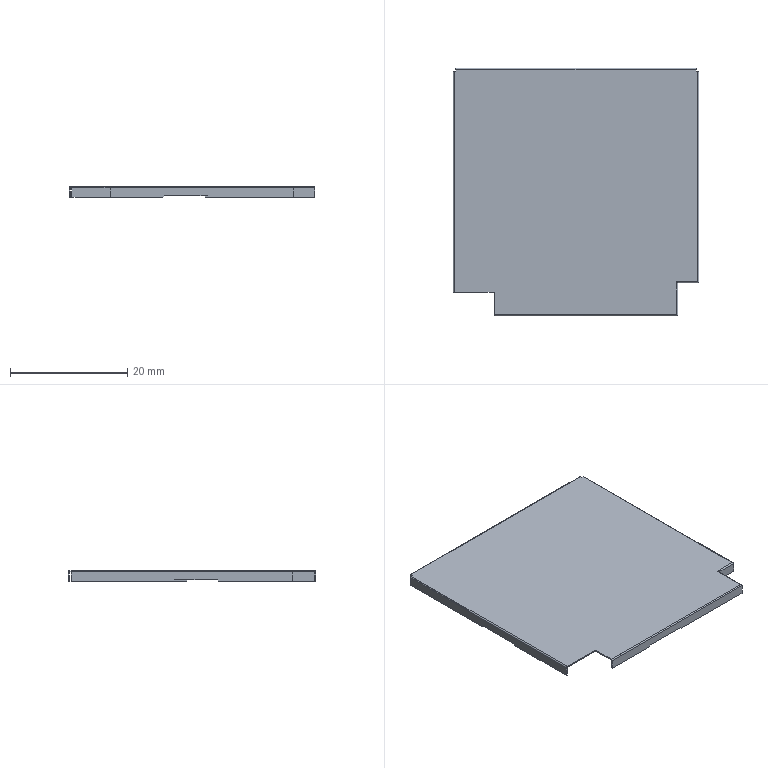Part | Creo | 1 solid | 45 faces | box 41.9 x 42.2 x 1.8 mm | volume 390.663 mm3 | plane 39 | cylinder 6 | commonest cylinder face diameters 0.4 x6
STEP:
#1=CARTESIAN_POINT('',(0.,0.,0.));
#2=DIRECTION('',(0.,0.,1.));
#3=DIRECTION('',(1.,0.,0.));
#4=AXIS2_PLACEMENT_3D('',#1,#2,#3);
#5=CARTESIAN_POINT('',(6.9,0.1,1.8));
#6=VERTEX_POINT('',#5);
#7=CARTESIAN_POINT('',(6.9,3.9,1.8));
#8=VERTEX_POINT('',#7);
#9=CARTESIAN_POINT('',(6.9,0.1,1.8));
#10=DIRECTION('',(0.,1.,0.));
#11=VECTOR('',#10,3.8);
#12=LINE('',#9,#11);
#13=EDGE_CURVE('',#6,#8,#12,.T.);
#14=ORIENTED_EDGE('',*,*,#13,.T.);
#15=CARTESIAN_POINT('',(0.1,3.9,1.8));
#16=VERTEX_POINT('',#15);
#17=CARTESIAN_POINT('',(0.1,3.9,1.8));
#18=DIRECTION('',(1.,0.,0.));
#19=VECTOR('',#18,6.8);
#20=LINE('',#17,#19);
#21=EDGE_CURVE('',#16,#8,#20,.T.);
#22=ORIENTED_EDGE('',*,*,#21,.F.);
#23=CARTESIAN_POINT('',(0.1,41.6,1.8));
#24=VERTEX_POINT('',#23);
#25=CARTESIAN_POINT('',(0.1,41.6,1.8));
#26=DIRECTION('',(0.,-1.,0.));
#27=VECTOR('',#26,37.7);
#28=LINE('',#25,#27);
#29=EDGE_CURVE('',#24,#16,#28,.T.);
#30=ORIENTED_EDGE('',*,*,#29,.F.);
#31=CARTESIAN_POINT('',(0.4,41.6,1.8));
#32=VERTEX_POINT('',#31);
#33=CARTESIAN_POINT('',(0.1,41.6,1.8));
#34=DIRECTION('',(1.,0.,0.));
#35=VECTOR('',#34,0.3);
#36=LINE('',#33,#35);
#37=EDGE_CURVE('',#24,#32,#36,.T.);
#38=ORIENTED_EDGE('',*,*,#37,.T.);
#39=CARTESIAN_POINT('',(0.4,41.9,1.8));
#40=VERTEX_POINT('',#39);
#41=CARTESIAN_POINT('',(0.4,41.9,1.8));
#42=DIRECTION('',(0.,-1.,0.));
#43=VECTOR('',#42,0.3);
#44=LINE('',#41,#43);
#45=EDGE_CURVE('',#40,#32,#44,.T.);
#46=ORIENTED_EDGE('',*,*,#45,.F.);
#47=CARTESIAN_POINT('',(41.3,41.9,1.8));
#48=VERTEX_POINT('',#47);
#49=CARTESIAN_POINT('',(41.3,41.9,1.8));
#50=DIRECTION('',(-1.,0.,0.));
#51=VECTOR('',#50,40.9);
#52=LINE('',#49,#51);
#53=EDGE_CURVE('',#48,#40,#52,.T.);
#54=ORIENTED_EDGE('',*,*,#53,.F.);
#55=CARTESIAN_POINT('',(41.3,41.6,1.8));
#56=VERTEX_POINT('',#55);
#57=CARTESIAN_POINT('',(41.3,41.9,1.8));
#58=DIRECTION('',(0.,-1.,0.));
#59=VECTOR('',#58,0.3);
#60=LINE('',#57,#59);
#61=EDGE_CURVE('',#48,#56,#60,.T.);
#62=ORIENTED_EDGE('',*,*,#61,.T.);
#63=CARTESIAN_POINT('',(41.6,41.6,1.8));
#64=VERTEX_POINT('',#63);
#65=CARTESIAN_POINT('',(41.6,41.6,1.8));
#66=DIRECTION('',(-1.,0.,0.));
#67=VECTOR('',#66,0.3);
#68=LINE('',#65,#67);
#69=EDGE_CURVE('',#64,#56,#68,.T.);
#70=ORIENTED_EDGE('',*,*,#69,.F.);
#71=CARTESIAN_POINT('',(41.6,5.7,1.8));
#72=VERTEX_POINT('',#71);
#73=CARTESIAN_POINT('',(41.6,5.7,1.8));
#74=DIRECTION('',(0.,1.,0.));
#75=VECTOR('',#74,35.9);
#76=LINE('',#73,#75);
#77=EDGE_CURVE('',#72,#64,#76,.T.);
#78=ORIENTED_EDGE('',*,*,#77,.F.);
#79=CARTESIAN_POINT('',(38.,5.7,1.8));
#80=VERTEX_POINT('',#79);
#81=CARTESIAN_POINT('',(38.,5.7,1.8));
#82=DIRECTION('',(1.,0.,0.));
#83=VECTOR('',#82,3.6);
#84=LINE('',#81,#83);
#85=EDGE_CURVE('',#80,#72,#84,.T.);
#86=ORIENTED_EDGE('',*,*,#85,.F.);
#87=CARTESIAN_POINT('',(38.,0.1,1.8));
#88=VERTEX_POINT('',#87);
#89=CARTESIAN_POINT('',(38.,0.1,1.8));
#90=DIRECTION('',(0.,1.,0.));
#91=VECTOR('',#90,5.6);
#92=LINE('',#89,#91);
#93=EDGE_CURVE('',#88,#80,#92,.T.);
#94=ORIENTED_EDGE('',*,*,#93,.F.);
#95=CARTESIAN_POINT('',(6.9,0.1,1.8));
#96=DIRECTION('',(1.,0.,0.));
#97=VECTOR('',#96,31.1);
#98=LINE('',#95,#97);
#99=EDGE_CURVE('',#6,#88,#98,.T.);
#100=ORIENTED_EDGE('',*,*,#99,.F.);
#101=EDGE_LOOP('',(#14,#22,#30,#38,#46,#54,#62,#70,#78,#86,#94,#100));
#102=FACE_OUTER_BOUND('',#101,.F.);
#103=CARTESIAN_POINT('',(0.,0.,1.8));
#104=DIRECTION('',(0.,0.,1.));
#105=DIRECTION('',(1.,0.,0.));
#106=AXIS2_PLACEMENT_3D('',#103,#104,#105);
#107=PLANE('',#106);
#108=ADVANCED_FACE('',(#102),#107,.T.);
#109=CARTESIAN_POINT('',(6.9,-0.1,0.));
#110=VERTEX_POINT('',#109);
#111=CARTESIAN_POINT('',(6.9,0.1,0.));
#112=VERTEX_POINT('',#111);
#113=CARTESIAN_POINT('',(6.9,-0.1,0.));
#114=DIRECTION('',(0.,1.,0.));
#115=VECTOR('',#114,0.2);
#116=LINE('',#113,#115);
#117=EDGE_CURVE('',#110,#112,#116,.T.);
#118=ORIENTED_EDGE('',*,*,#117,.T.);
#119=CARTESIAN_POINT('',(6.9,0.1,1.6));
#120=VERTEX_POINT('',#119);
#121=CARTESIAN_POINT('',(6.9,0.1,0.));
#122=DIRECTION('',(0.,0.,1.));
#123=VECTOR('',#122,1.6);
#124=LINE('',#121,#123);
#125=EDGE_CURVE('',#112,#120,#124,.T.);
#126=ORIENTED_EDGE('',*,*,#125,.T.);
#127=CARTESIAN_POINT('',(6.9,3.9,1.6));
#128=VERTEX_POINT('',#127);
#129=CARTESIAN_POINT('',(6.9,0.1,1.6));
#130=DIRECTION('',(0.,1.,0.));
#131=VECTOR('',#130,3.8);
#132=LINE('',#129,#131);
#133=EDGE_CURVE('',#120,#128,#132,.T.);
#134=ORIENTED_EDGE('',*,*,#133,.T.);
#135=CARTESIAN_POINT('',(6.9,3.9,1.8));
#136=DIRECTION('',(0.,0.,-1.));
#137=VECTOR('',#136,0.2);
#138=LINE('',#135,#137);
#139=EDGE_CURVE('',#8,#128,#138,.T.);
#140=ORIENTED_EDGE('',*,*,#139,.F.);
#141=ORIENTED_EDGE('',*,*,#13,.F.);
#142=CARTESIAN_POINT('',(6.9,-0.1,1.6));
#143=VERTEX_POINT('',#142);
#144=CARTESIAN_POINT('',(6.9,0.1,1.6));
#145=DIRECTION('',(1.,0.,0.));
#146=DIRECTION('',(0.,0.,1.));
#147=AXIS2_PLACEMENT_3D('',#144,#145,#146);
#148=CIRCLE('',#147,0.2);
#149=EDGE_CURVE('',#6,#143,#148,.T.);
#150=ORIENTED_EDGE('',*,*,#149,.T.);
#151=CARTESIAN_POINT('',(6.9,-0.1,0.));
#152=DIRECTION('',(0.,0.,1.));
#153=VECTOR('',#152,1.6);
#154=LINE('',#151,#153);
#155=EDGE_CURVE('',#110,#143,#154,.T.);
#156=ORIENTED_EDGE('',*,*,#155,.F.);
#157=EDGE_LOOP('',(#118,#126,#134,#140,#141,#150,#156));
#158=FACE_OUTER_BOUND('',#157,.F.);
#159=CARTESIAN_POINT('',(6.9,-0.1,1.8));
#160=DIRECTION('',(1.,0.,0.));
#161=DIRECTION('',(0.,1.,0.));
#162=AXIS2_PLACEMENT_3D('',#159,#160,#161);
#163=PLANE('',#162);
#164=ADVANCED_FACE('',(#158),#163,.F.);
#165=ORIENTED_EDGE('',*,*,#117,.F.);
#166=CARTESIAN_POINT('',(15.878,-0.1,0.));
#167=VERTEX_POINT('',#166);
#168=CARTESIAN_POINT('',(6.9,-0.1,0.));
#169=DIRECTION('',(1.,0.,0.));
#170=VECTOR('',#169,8.978);
#171=LINE('',#168,#170);
#172=EDGE_CURVE('',#110,#167,#171,.T.);
#173=ORIENTED_EDGE('',*,*,#172,.T.);
#174=CARTESIAN_POINT('',(15.878,0.1,0.));
#175=VERTEX_POINT('',#174);
#176=CARTESIAN_POINT('',(15.878,0.1,0.));
#177=DIRECTION('',(0.,-1.,0.));
#178=VECTOR('',#177,0.2);
#179=LINE('',#176,#178);
#180=EDGE_CURVE('',#175,#167,#179,.T.);
#181=ORIENTED_EDGE('',*,*,#180,.F.);
#182=CARTESIAN_POINT('',(6.9,0.1,0.));
#183=DIRECTION('',(1.,0.,0.));
#184=VECTOR('',#183,8.978);
#185=LINE('',#182,#184);
#186=EDGE_CURVE('',#112,#175,#185,.T.);
#187=ORIENTED_EDGE('',*,*,#186,.F.);
#188=EDGE_LOOP('',(#165,#173,#181,#187));
#189=FACE_OUTER_BOUND('',#188,.F.);
#190=CARTESIAN_POINT('',(0.,0.,0.));
#191=DIRECTION('',(0.,0.,1.));
#192=DIRECTION('',(1.,0.,0.));
#193=AXIS2_PLACEMENT_3D('',#190,#191,#192);
#194=PLANE('',#193);
#195=ADVANCED_FACE('',(#189),#194,.F.);
#196=ORIENTED_EDGE('',*,*,#155,.T.);
#197=CARTESIAN_POINT('',(38.2,-0.1,1.6));
#198=VERTEX_POINT('',#197);
#199=CARTESIAN_POINT('',(38.2,-0.1,1.6));
#200=DIRECTION('',(-1.,0.,0.));
#201=VECTOR('',#200,31.3);
#202=LINE('',#199,#201);
#203=EDGE_CURVE('',#198,#143,#202,.T.);
#204=ORIENTED_EDGE('',*,*,#203,.F.);
#205=CARTESIAN_POINT('',(38.2,-0.1,0.));
#206=VERTEX_POINT('',#205);
#207=CARTESIAN_POINT('',(38.2,-0.1,0.));
#208=DIRECTION('',(0.,0.,1.));
#209=VECTOR('',#208,1.6);
#210=LINE('',#207,#209);
#211=EDGE_CURVE('',#206,#198,#210,.T.);
#212=ORIENTED_EDGE('',*,*,#211,.F.);
#213=CARTESIAN_POINT('',(23.678,-0.1,0.));
#214=VERTEX_POINT('',#213);
#215=CARTESIAN_POINT('',(23.678,-0.1,0.));
#216=DIRECTION('',(1.,0.,0.));
#217=VECTOR('',#216,14.522);
#218=LINE('',#215,#217);
#219=EDGE_CURVE('',#214,#206,#218,.T.);
#220=ORIENTED_EDGE('',*,*,#219,.F.);
#221=CARTESIAN_POINT('',(23.428,-0.1,0.25));
#222=VERTEX_POINT('',#221);
#223=CARTESIAN_POINT('',(23.678,-0.1,0.));
#224=DIRECTION('',(-0.7071,0.,0.7071));
#225=VECTOR('',#224,0.3536);
#226=LINE('',#223,#225);
#227=EDGE_CURVE('',#214,#222,#226,.T.);
#228=ORIENTED_EDGE('',*,*,#227,.T.);
#229=CARTESIAN_POINT('',(16.128,-0.1,0.25));
#230=VERTEX_POINT('',#229);
#231=CARTESIAN_POINT('',(16.128,-0.1,0.25));
#232=DIRECTION('',(1.,0.,0.));
#233=VECTOR('',#232,7.3);
#234=LINE('',#231,#233);
#235=EDGE_CURVE('',#230,#222,#234,.T.);
#236=ORIENTED_EDGE('',*,*,#235,.F.);
#237=CARTESIAN_POINT('',(16.128,-0.1,0.25));
#238=DIRECTION('',(-0.7071,0.,-0.7071));
#239=VECTOR('',#238,0.3536);
#240=LINE('',#237,#239);
#241=EDGE_CURVE('',#230,#167,#240,.T.);
#242=ORIENTED_EDGE('',*,*,#241,.T.);
#243=ORIENTED_EDGE('',*,*,#172,.F.);
#244=EDGE_LOOP('',(#196,#204,#212,#220,#228,#236,#242,#243));
#245=FACE_OUTER_BOUND('',#244,.F.);
#246=CARTESIAN_POINT('',(-0.1,-0.1,0.));
#247=DIRECTION('',(0.,-1.,0.));
#248=DIRECTION('',(1.,0.,0.));
#249=AXIS2_PLACEMENT_3D('',#246,#247,#248);
#250=PLANE('',#249);
#251=ADVANCED_FACE('',(#245),#250,.T.);
#252=ORIENTED_EDGE('',*,*,#149,.F.);
#253=ORIENTED_EDGE('',*,*,#99,.T.);
#254=CARTESIAN_POINT('',(38.2,-0.1,1.6));
#255=CARTESIAN_POINT('',(38.2,-0.1,1.62));
#256=CARTESIAN_POINT('',(38.194,-0.09426,1.66));
#257=CARTESIAN_POINT('',(38.165,-0.06468,1.72));
#258=CARTESIAN_POINT('',(38.12,-0.02023,1.763));
#259=CARTESIAN_POINT('',(38.072,0.02774,1.79));
#260=CARTESIAN_POINT('',(38.026,0.07447,1.8));
#261=CARTESIAN_POINT('',(38.,0.1,1.8));
#262=B_SPLINE_CURVE_WITH_KNOTS('',3,(#254,#255,#256,#257,#258,#259,#260,#261),.UNSPECIFIED.,.F.,.F.,(4,1,1,1,1,4),(0.,0.2,0.4,0.6,0.8,1.),.UNSPECIFIED.);
#263=EDGE_CURVE('',#198,#88,#262,.T.);
#264=ORIENTED_EDGE('',*,*,#263,.F.);
#265=ORIENTED_EDGE('',*,*,#203,.T.);
#266=EDGE_LOOP('',(#252,#253,#264,#265));
#267=FACE_OUTER_BOUND('',#266,.F.);
#268=CARTESIAN_POINT('',(-55.792,0.1,1.6));
#269=DIRECTION('',(1.,0.,0.));
#270=DIRECTION('',(0.,0.,1.));
#271=AXIS2_PLACEMENT_3D('',#268,#269,#270);
#272=CYLINDRICAL_SURFACE('',#271,0.2);
#273=ADVANCED_FACE('',(#267),#272,.T.);
#274=CARTESIAN_POINT('',(38.2,5.5,1.6));
#275=VERTEX_POINT('',#274);
#276=CARTESIAN_POINT('',(38.2,5.5,1.6));
#277=DIRECTION('',(0.,-1.,0.));
#278=VECTOR('',#277,5.6);
#279=LINE('',#276,#278);
#280=EDGE_CURVE('',#275,#198,#279,.T.);
#281=ORIENTED_EDGE('',*,*,#280,.T.);
#282=ORIENTED_EDGE('',*,*,#263,.T.);
#283=ORIENTED_EDGE('',*,*,#93,.T.);
#284=CARTESIAN_POINT('',(38.2,5.5,1.6));
#285=CARTESIAN_POINT('',(38.2,5.5,1.62));
#286=CARTESIAN_POINT('',(38.194,5.506,1.66));
#287=CARTESIAN_POINT('',(38.165,5.535,1.72));
#288=CARTESIAN_POINT('',(38.12,5.58,1.763));
#289=CARTESIAN_POINT('',(38.072,5.628,1.79));
#290=CARTESIAN_POINT('',(38.026,5.674,1.8));
#291=CARTESIAN_POINT('',(38.,5.7,1.8));
#292=B_SPLINE_CURVE_WITH_KNOTS('',3,(#284,#285,#286,#287,#288,#289,#290,#291),.UNSPECIFIED.,.F.,.F.,(4,1,1,1,1,4),(0.,0.2,0.4,0.6,0.8,1.),.UNSPECIFIED.);
#293=EDGE_CURVE('',#275,#80,#292,.T.);
#294=ORIENTED_EDGE('',*,*,#293,.F.);
#295=EDGE_LOOP('',(#281,#282,#283,#294));
#296=FACE_OUTER_BOUND('',#295,.F.);
#297=CARTESIAN_POINT('',(38.,-56.156,1.6));
#298=DIRECTION('',(0.,1.,0.));
#299=DIRECTION('',(0.,0.,1.));
#300=AXIS2_PLACEMENT_3D('',#297,#298,#299);
#301=CYLINDRICAL_SURFACE('',#300,0.2);
#302=ADVANCED_FACE('',(#296),#301,.T.);
#303=ORIENTED_EDGE('',*,*,#280,.F.);
#304=CARTESIAN_POINT('',(38.2,5.5,0.));
#305=VERTEX_POINT('',#304);
#306=CARTESIAN_POINT('',(38.2,5.5,0.));
#307=DIRECTION('',(0.,0.,1.));
#308=VECTOR('',#307,1.6);
#309=LINE('',#306,#308);
#310=EDGE_CURVE('',#305,#275,#309,.T.);
#311=ORIENTED_EDGE('',*,*,#310,.F.);
#312=CARTESIAN_POINT('',(38.2,-0.1,0.));
#313=DIRECTION('',(0.,1.,0.));
#314=VECTOR('',#313,5.6);
#315=LINE('',#312,#314);
#316=EDGE_CURVE('',#206,#305,#315,.T.);
#317=ORIENTED_EDGE('',*,*,#316,.F.);
#318=ORIENTED_EDGE('',*,*,#211,.T.);
#319=EDGE_LOOP('',(#303,#311,#317,#318));
#320=FACE_OUTER_BOUND('',#319,.F.);
#321=CARTESIAN_POINT('',(38.2,-0.1,0.));
#322=DIRECTION('',(1.,0.,0.));
#323=DIRECTION('',(0.,1.,0.));
#324=AXIS2_PLACEMENT_3D('',#321,#322,#323);
#325=PLANE('',#324);
#326=ADVANCED_FACE('',(#320),#325,.T.);
#327=CARTESIAN_POINT('',(41.8,5.5,1.6));
#328=VERTEX_POINT('',#327);
#329=CARTESIAN_POINT('',(41.8,5.5,1.6));
#330=DIRECTION('',(-1.,0.,0.));
#331=VECTOR('',#330,3.6);
#332=LINE('',#329,#331);
#333=EDGE_CURVE('',#328,#275,#332,.T.);
#334=ORIENTED_EDGE('',*,*,#333,.F.);
#335=CARTESIAN_POINT('',(41.8,5.5,0.));
#336=VERTEX_POINT('',#335);
#337=CARTESIAN_POINT('',(41.8,5.5,0.));
#338=DIRECTION('',(0.,0.,1.));
#339=VECTOR('',#338,1.6);
#340=LINE('',#337,#339);
#341=EDGE_CURVE('',#336,#328,#340,.T.);
#342=ORIENTED_EDGE('',*,*,#341,.F.);
#343=CARTESIAN_POINT('',(38.2,5.5,0.));
#344=DIRECTION('',(1.,0.,0.));
#345=VECTOR('',#344,3.6);
#346=LINE('',#343,#345);
#347=EDGE_CURVE('',#305,#336,#346,.T.);
#348=ORIENTED_EDGE('',*,*,#347,.F.);
#349=ORIENTED_EDGE('',*,*,#310,.T.);
#350=EDGE_LOOP('',(#334,#342,#348,#349));
#351=FACE_OUTER_BOUND('',#350,.F.);
#352=CARTESIAN_POINT('',(38.2,5.5,0.));
#353=DIRECTION('',(0.,-1.,0.));
#354=DIRECTION('',(1.,0.,0.));
#355=AXIS2_PLACEMENT_3D('',#352,#353,#354);
#356=PLANE('',#355);
#357=ADVANCED_FACE('',(#351),#356,.T.);
#358=ORIENTED_EDGE('',*,*,#333,.T.);
#359=ORIENTED_EDGE('',*,*,#293,.T.);
#360=ORIENTED_EDGE('',*,*,#85,.T.);
#361=CARTESIAN_POINT('',(41.8,5.5,1.6));
#362=CARTESIAN_POINT('',(41.8,5.5,1.62));
#363=CARTESIAN_POINT('',(41.794,5.506,1.66));
#364=CARTESIAN_POINT('',(41.765,5.535,1.72));
#365=CARTESIAN_POINT('',(41.72,5.58,1.763));
#366=CARTESIAN_POINT('',(41.672,5.628,1.79));
#367=CARTESIAN_POINT('',(41.626,5.674,1.8));
#368=CARTESIAN_POINT('',(41.6,5.7,1.8));
#369=B_SPLINE_CURVE_WITH_KNOTS('',3,(#361,#362,#363,#364,#365,#366,#367,#368),.UNSPECIFIED.,.F.,.F.,(4,1,1,1,1,4),(0.,0.2,0.4,0.6,0.8,1.),.UNSPECIFIED.);
#370=EDGE_CURVE('',#328,#72,#369,.T.);
#371=ORIENTED_EDGE('',*,*,#370,.F.);
#372=EDGE_LOOP('',(#358,#359,#360,#371));
#373=FACE_OUTER_BOUND('',#372,.F.);
#374=CARTESIAN_POINT('',(-47.321,5.7,1.6));
#375=DIRECTION('',(1.,0.,0.));
#376=DIRECTION('',(0.,0.,1.));
#377=AXIS2_PLACEMENT_3D('',#374,#375,#376);
#378=CYLINDRICAL_SURFACE('',#377,0.2);
#379=ADVANCED_FACE('',(#373),#378,.T.);
#380=CARTESIAN_POINT('',(41.8,41.6,1.6));
#381=VERTEX_POINT('',#380);
#382=CARTESIAN_POINT('',(41.6,41.6,1.6));
#383=DIRECTION('',(0.,-1.,0.));
#384=DIRECTION('',(1.,0.,0.));
#385=AXIS2_PLACEMENT_3D('',#382,#383,#384);
#386=CIRCLE('',#385,0.2);
#387=EDGE_CURVE('',#381,#64,#386,.T.);
#388=ORIENTED_EDGE('',*,*,#387,.F.);
#389=CARTESIAN_POINT('',(41.8,41.6,1.6));
#390=DIRECTION('',(0.,-1.,0.));
#391=VECTOR('',#390,36.1);
#392=LINE('',#389,#391);
#393=EDGE_CURVE('',#381,#328,#392,.T.);
#394=ORIENTED_EDGE('',*,*,#393,.T.);
#395=ORIENTED_EDGE('',*,*,#370,.T.);
#396=ORIENTED_EDGE('',*,*,#77,.T.);
#397=EDGE_LOOP('',(#388,#394,#395,#396));
#398=FACE_OUTER_BOUND('',#397,.F.);
#399=CARTESIAN_POINT('',(41.6,-56.156,1.6));
#400=DIRECTION('',(0.,1.,0.));
#401=DIRECTION('',(0.,0.,1.));
#402=AXIS2_PLACEMENT_3D('',#399,#400,#401);
#403=CYLINDRICAL_SURFACE('',#402,0.2);
#404=ADVANCED_FACE('',(#398),#403,.T.);
#405=CARTESIAN_POINT('',(41.8,41.6,0.));
#406=VERTEX_POINT('',#405);
#407=CARTESIAN_POINT('',(41.6,41.6,0.));
#408=VERTEX_POINT('',#407);
#409=CARTESIAN_POINT('',(41.8,41.6,0.));
#410=DIRECTION('',(-1.,0.,0.));
#411=VECTOR('',#410,0.2);
#412=LINE('',#409,#411);
#413=EDGE_CURVE('',#406,#408,#412,.T.);
#414=ORIENTED_EDGE('',*,*,#413,.F.);
#415=CARTESIAN_POINT('',(41.8,41.6,0.));
#416=DIRECTION('',(0.,0.,1.));
#417=VECTOR('',#416,1.6);
#418=LINE('',#415,#417);
#419=EDGE_CURVE('',#406,#381,#418,.T.);
#420=ORIENTED_EDGE('',*,*,#419,.T.);
#421=ORIENTED_EDGE('',*,*,#387,.T.);
#422=ORIENTED_EDGE('',*,*,#69,.T.);
#423=CARTESIAN_POINT('',(41.3,41.6,1.6));
#424=VERTEX_POINT('',#423);
#425=CARTESIAN_POINT('',(41.3,41.6,1.8));
#426=DIRECTION('',(0.,0.,-1.));
#427=VECTOR('',#426,0.2);
#428=LINE('',#425,#427);
#429=EDGE_CURVE('',#56,#424,#428,.T.);
#430=ORIENTED_EDGE('',*,*,#429,.T.);
#431=CARTESIAN_POINT('',(41.6,41.6,1.6));
#432=VERTEX_POINT('',#431);
#433=CARTESIAN_POINT('',(41.6,41.6,1.6));
#434=DIRECTION('',(-1.,0.,0.));
#435=VECTOR('',#434,0.3);
#436=LINE('',#433,#435);
#437=EDGE_CURVE('',#432,#424,#436,.T.);
#438=ORIENTED_EDGE('',*,*,#437,.F.);
#439=CARTESIAN_POINT('',(41.6,41.6,0.));
#440=DIRECTION('',(0.,0.,1.));
#441=VECTOR('',#440,1.6);
#442=LINE('',#439,#441);
#443=EDGE_CURVE('',#408,#432,#442,.T.);
#444=ORIENTED_EDGE('',*,*,#443,.F.);
#445=EDGE_LOOP('',(#414,#420,#421,#422,#430,#438,#444));
#446=FACE_OUTER_BOUND('',#445,.F.);
#447=CARTESIAN_POINT('',(41.3,41.6,1.8));
#448=DIRECTION('',(0.,-1.,0.));
#449=DIRECTION('',(1.,0.,0.));
#450=AXIS2_PLACEMENT_3D('',#447,#448,#449);
#451=PLANE('',#450);
#452=ADVANCED_FACE('',(#446),#451,.F.);
#453=CARTESIAN_POINT('',(41.8,22.,0.));
#454=VERTEX_POINT('',#453);
#455=CARTESIAN_POINT('',(41.6,22.,0.));
#456=VERTEX_POINT('',#455);
#457=CARTESIAN_POINT('',(41.8,22.,0.));
#458=DIRECTION('',(-1.,0.,0.));
#459=VECTOR('',#458,0.2);
#460=LINE('',#457,#459);
#461=EDGE_CURVE('',#454,#456,#460,.T.);
#462=ORIENTED_EDGE('',*,*,#461,.F.);
#463=CARTESIAN_POINT('',(41.8,22.,0.));
#464=DIRECTION('',(0.,1.,0.));
#465=VECTOR('',#464,19.6);
#466=LINE('',#463,#465);
#467=EDGE_CURVE('',#454,#406,#466,.T.);
#468=ORIENTED_EDGE('',*,*,#467,.T.);
#469=ORIENTED_EDGE('',*,*,#413,.T.);
#470=CARTESIAN_POINT('',(41.6,22.,0.));
#471=DIRECTION('',(0.,1.,0.));
#472=VECTOR('',#471,19.6);
#473=LINE('',#470,#472);
#474=EDGE_CURVE('',#456,#408,#473,.T.);
#475=ORIENTED_EDGE('',*,*,#474,.F.);
#476=EDGE_LOOP('',(#462,#468,#469,#475));
#477=FACE_OUTER_BOUND('',#476,.F.);
#478=CARTESIAN_POINT('',(0.,0.,0.));
#479=DIRECTION('',(0.,0.,1.));
#480=DIRECTION('',(1.,0.,0.));
#481=AXIS2_PLACEMENT_3D('',#478,#479,#480);
#482=PLANE('',#481);
#483=ADVANCED_FACE('',(#477),#482,.F.);
#484=CARTESIAN_POINT('',(41.6,21.75,0.25));
#485=VERTEX_POINT('',#484);
#486=CARTESIAN_POINT('',(41.6,21.75,0.25));
#487=DIRECTION('',(0.,0.7071,-0.7071));
#488=VECTOR('',#487,0.3536);
#489=LINE('',#486,#488);
#490=EDGE_CURVE('',#485,#456,#489,.T.);
#491=ORIENTED_EDGE('',*,*,#490,.F.);
#492=CARTESIAN_POINT('',(41.8,21.75,0.25));
#493=VERTEX_POINT('',#492);
#494=CARTESIAN_POINT('',(41.8,21.75,0.25));
#495=DIRECTION('',(-1.,0.,0.));
#496=VECTOR('',#495,0.2);
#497=LINE('',#494,#496);
#498=EDGE_CURVE('',#493,#485,#497,.T.);
#499=ORIENTED_EDGE('',*,*,#498,.F.);
#500=CARTESIAN_POINT('',(41.8,22.,0.));
#501=DIRECTION('',(0.,-0.7071,0.7071));
#502=VECTOR('',#501,0.3536);
#503=LINE('',#500,#502);
#504=EDGE_CURVE('',#454,#493,#503,.T.);
#505=ORIENTED_EDGE('',*,*,#504,.F.);
#506=ORIENTED_EDGE('',*,*,#461,.T.);
#507=EDGE_LOOP('',(#491,#499,#505,#506));
#508=FACE_OUTER_BOUND('',#507,.F.);
#509=CARTESIAN_POINT('',(41.7,21.875,0.125));
#510=DIRECTION('',(0.,-0.7071,-0.7071));
#511=DIRECTION('',(0.,-0.7071,0.7071));
#512=AXIS2_PLACEMENT_3D('',#509,#510,#511);
#513=PLANE('',#512);
#514=ADVANCED_FACE('',(#508),#513,.T.);
#515=CARTESIAN_POINT('',(41.6,14.2,0.));
#516=VERTEX_POINT('',#515);
#517=CARTESIAN_POINT('',(41.6,14.45,0.25));
#518=VERTEX_POINT('',#517);
#519=CARTESIAN_POINT('',(41.6,14.2,0.));
#520=DIRECTION('',(0.,0.7071,0.7071));
#521=VECTOR('',#520,0.3536);
#522=LINE('',#519,#521);
#523=EDGE_CURVE('',#516,#518,#522,.T.);
#524=ORIENTED_EDGE('',*,*,#523,.T.);
#525=CARTESIAN_POINT('',(41.6,14.45,0.25));
#526=DIRECTION('',(0.,1.,0.));
#527=VECTOR('',#526,7.3);
#528=LINE('',#525,#527);
#529=EDGE_CURVE('',#518,#485,#528,.T.);
#530=ORIENTED_EDGE('',*,*,#529,.T.);
#531=ORIENTED_EDGE('',*,*,#490,.T.);
#532=ORIENTED_EDGE('',*,*,#474,.T.);
#533=ORIENTED_EDGE('',*,*,#443,.T.);
#534=CARTESIAN_POINT('',(41.6,5.7,1.6));
#535=VERTEX_POINT('',#534);
#536=CARTESIAN_POINT('',(41.6,5.7,1.6));
#537=DIRECTION('',(0.,1.,0.));
#538=VECTOR('',#537,35.9);
#539=LINE('',#536,#538);
#540=EDGE_CURVE('',#535,#432,#539,.T.);
#541=ORIENTED_EDGE('',*,*,#540,.F.);
#542=CARTESIAN_POINT('',(41.6,5.7,0.));
#543=VERTEX_POINT('',#542);
#544=CARTESIAN_POINT('',(41.6,5.7,0.));
#545=DIRECTION('',(0.,0.,1.));
#546=VECTOR('',#545,1.6);
#547=LINE('',#544,#546);
#548=EDGE_CURVE('',#543,#535,#547,.T.);
#549=ORIENTED_EDGE('',*,*,#548,.F.);
#550=CARTESIAN_POINT('',(41.6,5.7,0.));
#551=DIRECTION('',(0.,1.,0.));
#552=VECTOR('',#551,8.5);
#553=LINE('',#550,#552);
#554=EDGE_CURVE('',#543,#516,#553,.T.);
#555=ORIENTED_EDGE('',*,*,#554,.T.);
#556=EDGE_LOOP('',(#524,#530,#531,#532,#533,#541,#549,#555));
#557=FACE_OUTER_BOUND('',#556,.F.);
#558=CARTESIAN_POINT('',(41.6,5.5,0.));
#559=DIRECTION('',(1.,0.,0.));
#560=DIRECTION('',(0.,1.,0.));
#561=AXIS2_PLACEMENT_3D('',#558,#559,#560);
#562=PLANE('',#561);
#563=ADVANCED_FACE('',(#557),#562,.F.);
#564=CARTESIAN_POINT('',(41.8,14.45,0.25));
#565=VERTEX_POINT('',#564);
#566=CARTESIAN_POINT('',(41.8,14.2,0.));
#567=VERTEX_POINT('',#566);
#568=CARTESIAN_POINT('',(41.8,14.45,0.25));
#569=DIRECTION('',(0.,-0.7071,-0.7071));
#570=VECTOR('',#569,0.3536);
#571=LINE('',#568,#570);
#572=EDGE_CURVE('',#565,#567,#571,.T.);
#573=ORIENTED_EDGE('',*,*,#572,.F.);
#574=CARTESIAN_POINT('',(41.6,14.45,0.25));
#575=DIRECTION('',(1.,0.,0.));
#576=VECTOR('',#575,0.2);
#577=LINE('',#574,#576);
#578=EDGE_CURVE('',#518,#565,#577,.T.);
#579=ORIENTED_EDGE('',*,*,#578,.F.);
#580=ORIENTED_EDGE('',*,*,#523,.F.);
#581=CARTESIAN_POINT('',(41.6,14.2,0.));
#582=DIRECTION('',(1.,0.,0.));
#583=VECTOR('',#582,0.2);
#584=LINE('',#581,#583);
#585=EDGE_CURVE('',#516,#567,#584,.T.);
#586=ORIENTED_EDGE('',*,*,#585,.T.);
#587=EDGE_LOOP('',(#573,#579,#580,#586));
#588=FACE_OUTER_BOUND('',#587,.F.);
#589=CARTESIAN_POINT('',(41.7,14.325,0.125));
#590=DIRECTION('',(0.,0.7071,-0.7071));
#591=DIRECTION('',(0.,0.7071,0.7071));
#592=AXIS2_PLACEMENT_3D('',#589,#590,#591);
#593=PLANE('',#592);
#594=ADVANCED_FACE('',(#588),#593,.T.);
#595=ORIENTED_EDGE('',*,*,#572,.T.);
#596=CARTESIAN_POINT('',(41.8,5.5,0.));
#597=DIRECTION('',(0.,1.,0.));
#598=VECTOR('',#597,8.7);
#599=LINE('',#596,#598);
#600=EDGE_CURVE('',#336,#567,#599,.T.);
#601=ORIENTED_EDGE('',*,*,#600,.F.);
#602=ORIENTED_EDGE('',*,*,#341,.T.);
#603=ORIENTED_EDGE('',*,*,#393,.F.);
#604=ORIENTED_EDGE('',*,*,#419,.F.);
#605=ORIENTED_EDGE('',*,*,#467,.F.);
#606=ORIENTED_EDGE('',*,*,#504,.T.);
#607=CARTESIAN_POINT('',(41.8,14.45,0.25));
#608=DIRECTION('',(0.,1.,0.));
#609=VECTOR('',#608,7.3);
#610=LINE('',#607,#609);
#611=EDGE_CURVE('',#565,#493,#610,.T.);
#612=ORIENTED_EDGE('',*,*,#611,.F.);
#613=EDGE_LOOP('',(#595,#601,#602,#603,#604,#605,#606,#612));
#614=FACE_OUTER_BOUND('',#613,.F.);
#615=CARTESIAN_POINT('',(41.8,5.5,0.));
#616=DIRECTION('',(1.,0.,0.));
#617=DIRECTION('',(0.,1.,0.));
#618=AXIS2_PLACEMENT_3D('',#615,#616,#617);
#619=PLANE('',#618);
#620=ADVANCED_FACE('',(#614),#619,.T.);
#621=CARTESIAN_POINT('',(23.678,0.1,0.));
#622=VERTEX_POINT('',#621);
#623=CARTESIAN_POINT('',(23.678,-0.1,0.));
#624=DIRECTION('',(0.,1.,0.));
#625=VECTOR('',#624,0.2);
#626=LINE('',#623,#625);
#627=EDGE_CURVE('',#214,#622,#626,.T.);
#628=ORIENTED_EDGE('',*,*,#627,.F.);
#629=ORIENTED_EDGE('',*,*,#219,.T.);
#630=ORIENTED_EDGE('',*,*,#316,.T.);
#631=ORIENTED_EDGE('',*,*,#347,.T.);
#632=ORIENTED_EDGE('',*,*,#600,.T.);
#633=ORIENTED_EDGE('',*,*,#585,.F.);
#634=ORIENTED_EDGE('',*,*,#554,.F.);
#635=CARTESIAN_POINT('',(38.,5.7,0.));
#636=VERTEX_POINT('',#635);
#637=CARTESIAN_POINT('',(38.,5.7,0.));
#638=DIRECTION('',(1.,0.,0.));
#639=VECTOR('',#638,3.6);
#640=LINE('',#637,#639);
#641=EDGE_CURVE('',#636,#543,#640,.T.);
#642=ORIENTED_EDGE('',*,*,#641,.F.);
#643=CARTESIAN_POINT('',(38.,0.1,0.));
#644=VERTEX_POINT('',#643);
#645=CARTESIAN_POINT('',(38.,0.1,0.));
#646=DIRECTION('',(0.,1.,0.));
#647=VECTOR('',#646,5.6);
#648=LINE('',#645,#647);
#649=EDGE_CURVE('',#644,#636,#648,.T.);
#650=ORIENTED_EDGE('',*,*,#649,.F.);
#651=CARTESIAN_POINT('',(23.678,0.1,0.));
#652=DIRECTION('',(1.,0.,0.));
#653=VECTOR('',#652,14.322);
#654=LINE('',#651,#653);
#655=EDGE_CURVE('',#622,#644,#654,.T.);
#656=ORIENTED_EDGE('',*,*,#655,.F.);
#657=EDGE_LOOP('',(#628,#629,#630,#631,#632,#633,#634,#642,#650,#656));
#658=FACE_OUTER_BOUND('',#657,.F.);
#659=CARTESIAN_POINT('',(0.,0.,0.));
#660=DIRECTION('',(0.,0.,1.));
#661=DIRECTION('',(1.,0.,0.));
#662=AXIS2_PLACEMENT_3D('',#659,#660,#661);
#663=PLANE('',#662);
#664=ADVANCED_FACE('',(#658),#663,.F.);
#665=CARTESIAN_POINT('',(23.428,0.1,0.25));
#666=VERTEX_POINT('',#665);
#667=CARTESIAN_POINT('',(23.428,0.1,0.25));
#668=DIRECTION('',(0.7071,0.,-0.7071));
#669=VECTOR('',#668,0.3536);
#670=LINE('',#667,#669);
#671=EDGE_CURVE('',#666,#622,#670,.T.);
#672=ORIENTED_EDGE('',*,*,#671,.F.);
#673=CARTESIAN_POINT('',(23.428,-0.1,0.25));
#674=DIRECTION('',(0.,1.,0.));
#675=VECTOR('',#674,0.2);
#676=LINE('',#673,#675);
#677=EDGE_CURVE('',#222,#666,#676,.T.);
#678=ORIENTED_EDGE('',*,*,#677,.F.);
#679=ORIENTED_EDGE('',*,*,#227,.F.);
#680=ORIENTED_EDGE('',*,*,#627,.T.);
#681=EDGE_LOOP('',(#672,#678,#679,#680));
#682=FACE_OUTER_BOUND('',#681,.F.);
#683=CARTESIAN_POINT('',(23.553,0.,0.125));
#684=DIRECTION('',(-0.7071,0.,-0.7071));
#685=DIRECTION('',(-0.7071,0.,0.7071));
#686=AXIS2_PLACEMENT_3D('',#683,#684,#685);
#687=PLANE('',#686);
#688=ADVANCED_FACE('',(#682),#687,.T.);
#689=ORIENTED_EDGE('',*,*,#125,.F.);
#690=ORIENTED_EDGE('',*,*,#186,.T.);
#691=CARTESIAN_POINT('',(16.128,0.1,0.25));
#692=VERTEX_POINT('',#691);
#693=CARTESIAN_POINT('',(15.878,0.1,0.));
#694=DIRECTION('',(0.7071,0.,0.7071));
#695=VECTOR('',#694,0.3536);
#696=LINE('',#693,#695);
#697=EDGE_CURVE('',#175,#692,#696,.T.);
#698=ORIENTED_EDGE('',*,*,#697,.T.);
#699=CARTESIAN_POINT('',(16.128,0.1,0.25));
#700=DIRECTION('',(1.,0.,0.));
#701=VECTOR('',#700,7.3);
#702=LINE('',#699,#701);
#703=EDGE_CURVE('',#692,#666,#702,.T.);
#704=ORIENTED_EDGE('',*,*,#703,.T.);
#705=ORIENTED_EDGE('',*,*,#671,.T.);
#706=ORIENTED_EDGE('',*,*,#655,.T.);
#707=CARTESIAN_POINT('',(38.,0.1,1.6));
#708=VERTEX_POINT('',#707);
#709=CARTESIAN_POINT('',(38.,0.1,0.));
#710=DIRECTION('',(0.,0.,1.));
#711=VECTOR('',#710,1.6);
#712=LINE('',#709,#711);
#713=EDGE_CURVE('',#644,#708,#712,.T.);
#714=ORIENTED_EDGE('',*,*,#713,.T.);
#715=CARTESIAN_POINT('',(6.9,0.1,1.6));
#716=DIRECTION('',(1.,0.,0.));
#717=VECTOR('',#716,31.1);
#718=LINE('',#715,#717);
#719=EDGE_CURVE('',#120,#708,#718,.T.);
#720=ORIENTED_EDGE('',*,*,#719,.F.);
#721=EDGE_LOOP('',(#689,#690,#698,#704,#705,#706,#714,#720));
#722=FACE_OUTER_BOUND('',#721,.F.);
#723=CARTESIAN_POINT('',(-0.1,0.1,0.));
#724=DIRECTION('',(0.,-1.,0.));
#725=DIRECTION('',(1.,0.,0.));
#726=AXIS2_PLACEMENT_3D('',#723,#724,#725);
#727=PLANE('',#726);
#728=ADVANCED_FACE('',(#722),#727,.F.);
#729=ORIENTED_EDGE('',*,*,#241,.F.);
#730=CARTESIAN_POINT('',(16.128,0.1,0.25));
#731=DIRECTION('',(0.,-1.,0.));
#732=VECTOR('',#731,0.2);
#733=LINE('',#730,#732);
#734=EDGE_CURVE('',#692,#230,#733,.T.);
#735=ORIENTED_EDGE('',*,*,#734,.F.);
#736=ORIENTED_EDGE('',*,*,#697,.F.);
#737=ORIENTED_EDGE('',*,*,#180,.T.);
#738=EDGE_LOOP('',(#729,#735,#736,#737));
#739=FACE_OUTER_BOUND('',#738,.F.);
#740=CARTESIAN_POINT('',(16.003,0.,0.125));
#741=DIRECTION('',(0.7071,0.,-0.7071));
#742=DIRECTION('',(0.7071,0.,0.7071));
#743=AXIS2_PLACEMENT_3D('',#740,#741,#742);
#744=PLANE('',#743);
#745=ADVANCED_FACE('',(#739),#744,.T.);
#746=ORIENTED_EDGE('',*,*,#734,.T.);
#747=ORIENTED_EDGE('',*,*,#235,.T.);
#748=ORIENTED_EDGE('',*,*,#677,.T.);
#749=ORIENTED_EDGE('',*,*,#703,.F.);
#750=EDGE_LOOP('',(#746,#747,#748,#749));
#751=FACE_OUTER_BOUND('',#750,.F.);
#752=CARTESIAN_POINT('',(0.,0.,0.25));
#753=DIRECTION('',(0.,0.,-1.));
#754=DIRECTION('',(0.,1.,0.));
#755=AXIS2_PLACEMENT_3D('',#752,#753,#754);
#756=PLANE('',#755);
#757=ADVANCED_FACE('',(#751),#756,.T.);
#758=ORIENTED_EDGE('',*,*,#649,.T.);
#759=CARTESIAN_POINT('',(38.,5.7,1.6));
#760=VERTEX_POINT('',#759);
#761=CARTESIAN_POINT('',(38.,5.7,0.));
#762=DIRECTION('',(0.,0.,1.));
#763=VECTOR('',#762,1.6);
#764=LINE('',#761,#763);
#765=EDGE_CURVE('',#636,#760,#764,.T.);
#766=ORIENTED_EDGE('',*,*,#765,.T.);
#767=CARTESIAN_POINT('',(38.,0.1,1.6));
#768=DIRECTION('',(0.,1.,0.));
#769=VECTOR('',#768,5.6);
#770=LINE('',#767,#769);
#771=EDGE_CURVE('',#708,#760,#770,.T.);
#772=ORIENTED_EDGE('',*,*,#771,.F.);
#773=ORIENTED_EDGE('',*,*,#713,.F.);
#774=EDGE_LOOP('',(#758,#766,#772,#773));
#775=FACE_OUTER_BOUND('',#774,.F.);
#776=CARTESIAN_POINT('',(38.,-0.1,0.));
#777=DIRECTION('',(1.,0.,0.));
#778=DIRECTION('',(0.,1.,0.));
#779=AXIS2_PLACEMENT_3D('',#776,#777,#778);
#780=PLANE('',#779);
#781=ADVANCED_FACE('',(#775),#780,.F.);
#782=ORIENTED_EDGE('',*,*,#641,.T.);
#783=ORIENTED_EDGE('',*,*,#548,.T.);
#784=CARTESIAN_POINT('',(38.,5.7,1.6));
#785=DIRECTION('',(1.,0.,0.));
#786=VECTOR('',#785,3.6);
#787=LINE('',#784,#786);
#788=EDGE_CURVE('',#760,#535,#787,.T.);
#789=ORIENTED_EDGE('',*,*,#788,.F.);
#790=ORIENTED_EDGE('',*,*,#765,.F.);
#791=EDGE_LOOP('',(#782,#783,#789,#790));
#792=FACE_OUTER_BOUND('',#791,.F.);
#793=CARTESIAN_POINT('',(38.2,5.7,0.));
#794=DIRECTION('',(0.,-1.,0.));
#795=DIRECTION('',(1.,0.,0.));
#796=AXIS2_PLACEMENT_3D('',#793,#794,#795);
#797=PLANE('',#796);
#798=ADVANCED_FACE('',(#792),#797,.F.);
#799=ORIENTED_EDGE('',*,*,#133,.F.);
#800=ORIENTED_EDGE('',*,*,#719,.T.);
#801=ORIENTED_EDGE('',*,*,#771,.T.);
#802=ORIENTED_EDGE('',*,*,#788,.T.);
#803=ORIENTED_EDGE('',*,*,#540,.T.);
#804=ORIENTED_EDGE('',*,*,#437,.T.);
#805=CARTESIAN_POINT('',(41.3,41.9,1.6));
#806=VERTEX_POINT('',#805);
#807=CARTESIAN_POINT('',(41.3,41.9,1.6));
#808=DIRECTION('',(0.,-1.,0.));
#809=VECTOR('',#808,0.3);
#810=LINE('',#807,#809);
#811=EDGE_CURVE('',#806,#424,#810,.T.);
#812=ORIENTED_EDGE('',*,*,#811,.F.);
#813=CARTESIAN_POINT('',(0.4,41.9,1.6));
#814=VERTEX_POINT('',#813);
#815=CARTESIAN_POINT('',(41.3,41.9,1.6));
#816=DIRECTION('',(-1.,0.,0.));
#817=VECTOR('',#816,40.9);
#818=LINE('',#815,#817);
#819=EDGE_CURVE('',#806,#814,#818,.T.);
#820=ORIENTED_EDGE('',*,*,#819,.T.);
#821=CARTESIAN_POINT('',(0.4,41.6,1.6));
#822=VERTEX_POINT('',#821);
#823=CARTESIAN_POINT('',(0.4,41.9,1.6));
#824=DIRECTION('',(0.,-1.,0.));
#825=VECTOR('',#824,0.3);
#826=LINE('',#823,#825);
#827=EDGE_CURVE('',#814,#822,#826,.T.);
#828=ORIENTED_EDGE('',*,*,#827,.T.);
#829=CARTESIAN_POINT('',(0.1,41.6,1.6));
#830=VERTEX_POINT('',#829);
#831=CARTESIAN_POINT('',(0.1,41.6,1.6));
#832=DIRECTION('',(1.,0.,0.));
#833=VECTOR('',#832,0.3);
#834=LINE('',#831,#833);
#835=EDGE_CURVE('',#830,#822,#834,.T.);
#836=ORIENTED_EDGE('',*,*,#835,.F.);
#837=CARTESIAN_POINT('',(0.1,3.9,1.6));
#838=VERTEX_POINT('',#837);
#839=CARTESIAN_POINT('',(0.1,41.6,1.6));
#840=DIRECTION('',(0.,-1.,0.));
#841=VECTOR('',#840,37.7);
#842=LINE('',#839,#841);
#843=EDGE_CURVE('',#830,#838,#842,.T.);
#844=ORIENTED_EDGE('',*,*,#843,.T.);
#845=CARTESIAN_POINT('',(0.1,3.9,1.6));
#846=DIRECTION('',(1.,0.,0.));
#847=VECTOR('',#846,6.8);
#848=LINE('',#845,#847);
#849=EDGE_CURVE('',#838,#128,#848,.T.);
#850=ORIENTED_EDGE('',*,*,#849,.T.);
#851=EDGE_LOOP('',(#799,#800,#801,#802,#803,#804,#812,#820,#828,#836,#844,#850));
#852=FACE_OUTER_BOUND('',#851,.F.);
#853=CARTESIAN_POINT('',(0.,0.,1.6));
#854=DIRECTION('',(0.,0.,1.));
#855=DIRECTION('',(1.,0.,0.));
#856=AXIS2_PLACEMENT_3D('',#853,#854,#855);
#857=PLANE('',#856);
#858=ADVANCED_FACE('',(#852),#857,.F.);
#859=CARTESIAN_POINT('',(41.3,42.1,0.));
#860=VERTEX_POINT('',#859);
#861=CARTESIAN_POINT('',(41.3,41.9,0.));
#862=VERTEX_POINT('',#861);
#863=CARTESIAN_POINT('',(41.3,42.1,0.));
#864=DIRECTION('',(0.,-1.,0.));
#865=VECTOR('',#864,0.2);
#866=LINE('',#863,#865);
#867=EDGE_CURVE('',#860,#862,#866,.T.);
#868=ORIENTED_EDGE('',*,*,#867,.T.);
#869=CARTESIAN_POINT('',(41.3,41.9,0.));
#870=DIRECTION('',(0.,0.,1.));
#871=VECTOR('',#870,1.6);
#872=LINE('',#869,#871);
#873=EDGE_CURVE('',#862,#806,#872,.T.);
#874=ORIENTED_EDGE('',*,*,#873,.T.);
#875=ORIENTED_EDGE('',*,*,#811,.T.);
#876=ORIENTED_EDGE('',*,*,#429,.F.);
#877=ORIENTED_EDGE('',*,*,#61,.F.);
#878=CARTESIAN_POINT('',(41.3,42.1,1.6));
#879=VERTEX_POINT('',#878);
#880=CARTESIAN_POINT('',(41.3,41.9,1.6));
#881=DIRECTION('',(-1.,0.,0.));
#882=DIRECTION('',(0.,0.,1.));
#883=AXIS2_PLACEMENT_3D('',#880,#881,#882);
#884=CIRCLE('',#883,0.2);
#885=EDGE_CURVE('',#48,#879,#884,.T.);
#886=ORIENTED_EDGE('',*,*,#885,.T.);
#887=CARTESIAN_POINT('',(41.3,42.1,0.));
#888=DIRECTION('',(0.,0.,1.));
#889=VECTOR('',#888,1.6);
#890=LINE('',#887,#889);
#891=EDGE_CURVE('',#860,#879,#890,.T.);
#892=ORIENTED_EDGE('',*,*,#891,.F.);
#893=EDGE_LOOP('',(#868,#874,#875,#876,#877,#886,#892));
#894=FACE_OUTER_BOUND('',#893,.F.);
#895=CARTESIAN_POINT('',(41.3,42.1,1.8));
#896=DIRECTION('',(-1.,0.,0.));
#897=DIRECTION('',(0.,-1.,0.));
#898=AXIS2_PLACEMENT_3D('',#895,#896,#897);
#899=PLANE('',#898);
#900=ADVANCED_FACE('',(#894),#899,.F.);
#901=CARTESIAN_POINT('',(23.172,41.9,0.));
#902=VERTEX_POINT('',#901);
#903=CARTESIAN_POINT('',(23.172,42.1,0.));
#904=VERTEX_POINT('',#903);
#905=CARTESIAN_POINT('',(23.172,41.9,0.));
#906=DIRECTION('',(0.,1.,0.));
#907=VECTOR('',#906,0.2);
#908=LINE('',#905,#907);
#909=EDGE_CURVE('',#902,#904,#908,.T.);
#910=ORIENTED_EDGE('',*,*,#909,.F.);
#911=CARTESIAN_POINT('',(41.3,41.9,0.));
#912=DIRECTION('',(-1.,0.,0.));
#913=VECTOR('',#912,18.128);
#914=LINE('',#911,#913);
#915=EDGE_CURVE('',#862,#902,#914,.T.);
#916=ORIENTED_EDGE('',*,*,#915,.F.);
#917=ORIENTED_EDGE('',*,*,#867,.F.);
#918=CARTESIAN_POINT('',(41.3,42.1,0.));
#919=DIRECTION('',(-1.,0.,0.));
#920=VECTOR('',#919,18.128);
#921=LINE('',#918,#920);
#922=EDGE_CURVE('',#860,#904,#921,.T.);
#923=ORIENTED_EDGE('',*,*,#922,.T.);
#924=EDGE_LOOP('',(#910,#916,#917,#923));
#925=FACE_OUTER_BOUND('',#924,.F.);
#926=CARTESIAN_POINT('',(0.,0.,0.));
#927=DIRECTION('',(0.,0.,1.));
#928=DIRECTION('',(1.,0.,0.));
#929=AXIS2_PLACEMENT_3D('',#926,#927,#928);
#930=PLANE('',#929);
#931=ADVANCED_FACE('',(#925),#930,.F.);
#932=CARTESIAN_POINT('',(22.922,42.1,0.25));
#933=VERTEX_POINT('',#932);
#934=CARTESIAN_POINT('',(22.922,42.1,0.25));
#935=DIRECTION('',(0.7071,0.,-0.7071));
#936=VECTOR('',#935,0.3536);
#937=LINE('',#934,#936);
#938=EDGE_CURVE('',#933,#904,#937,.T.);
#939=ORIENTED_EDGE('',*,*,#938,.F.);
#940=CARTESIAN_POINT('',(22.922,41.9,0.25));
#941=VERTEX_POINT('',#940);
#942=CARTESIAN_POINT('',(22.922,41.9,0.25));
#943=DIRECTION('',(0.,1.,0.));
#944=VECTOR('',#943,0.2);
#945=LINE('',#942,#944);
#946=EDGE_CURVE('',#941,#933,#945,.T.);
#947=ORIENTED_EDGE('',*,*,#946,.F.);
#948=CARTESIAN_POINT('',(23.172,41.9,0.));
#949=DIRECTION('',(-0.7071,0.,0.7071));
#950=VECTOR('',#949,0.3536);
#951=LINE('',#948,#950);
#952=EDGE_CURVE('',#902,#941,#951,.T.);
#953=ORIENTED_EDGE('',*,*,#952,.F.);
#954=ORIENTED_EDGE('',*,*,#909,.T.);
#955=EDGE_LOOP('',(#939,#947,#953,#954));
#956=FACE_OUTER_BOUND('',#955,.F.);
#957=CARTESIAN_POINT('',(23.047,42.,0.125));
#958=DIRECTION('',(-0.7071,0.,-0.7071));
#959=DIRECTION('',(-0.7071,0.,0.7071));
#960=AXIS2_PLACEMENT_3D('',#957,#958,#959);
#961=PLANE('',#960);
#962=ADVANCED_FACE('',(#956),#961,.T.);
#963=ORIENTED_EDGE('',*,*,#938,.T.);
#964=ORIENTED_EDGE('',*,*,#922,.F.);
#965=ORIENTED_EDGE('',*,*,#891,.T.);
#966=CARTESIAN_POINT('',(0.4,42.1,1.6));
#967=VERTEX_POINT('',#966);
#968=CARTESIAN_POINT('',(0.4,42.1,1.6));
#969=DIRECTION('',(1.,0.,0.));
#970=VECTOR('',#969,40.9);
#971=LINE('',#968,#970);
#972=EDGE_CURVE('',#967,#879,#971,.T.);
#973=ORIENTED_EDGE('',*,*,#972,.F.);
#974=CARTESIAN_POINT('',(0.4,42.1,0.));
#975=VERTEX_POINT('',#974);
#976=CARTESIAN_POINT('',(0.4,42.1,0.));
#977=DIRECTION('',(0.,0.,1.));
#978=VECTOR('',#977,1.6);
#979=LINE('',#976,#978);
#980=EDGE_CURVE('',#975,#967,#979,.T.);
#981=ORIENTED_EDGE('',*,*,#980,.F.);
#982=CARTESIAN_POINT('',(15.372,42.1,0.));
#983=VERTEX_POINT('',#982);
#984=CARTESIAN_POINT('',(15.372,42.1,0.));
#985=DIRECTION('',(-1.,0.,0.));
#986=VECTOR('',#985,14.972);
#987=LINE('',#984,#986);
#988=EDGE_CURVE('',#983,#975,#987,.T.);
#989=ORIENTED_EDGE('',*,*,#988,.F.);
#990=CARTESIAN_POINT('',(15.622,42.1,0.25));
#991=VERTEX_POINT('',#990);
#992=CARTESIAN_POINT('',(15.372,42.1,0.));
#993=DIRECTION('',(0.7071,0.,0.7071));
#994=VECTOR('',#993,0.3536);
#995=LINE('',#992,#994);
#996=EDGE_CURVE('',#983,#991,#995,.T.);
#997=ORIENTED_EDGE('',*,*,#996,.T.);
#998=CARTESIAN_POINT('',(22.922,42.1,0.25));
#999=DIRECTION('',(-1.,0.,0.));
#1000=VECTOR('',#999,7.3);
#1001=LINE('',#998,#1000);
#1002=EDGE_CURVE('',#933,#991,#1001,.T.);
#1003=ORIENTED_EDGE('',*,*,#1002,.F.);
#1004=EDGE_LOOP('',(#963,#964,#965,#973,#981,#989,#997,#1003));
#1005=FACE_OUTER_BOUND('',#1004,.F.);
#1006=CARTESIAN_POINT('',(41.8,42.1,0.));
#1007=DIRECTION('',(0.,1.,0.));
#1008=DIRECTION('',(-1.,0.,0.));
#1009=AXIS2_PLACEMENT_3D('',#1006,#1007,#1008);
#1010=PLANE('',#1009);
#1011=ADVANCED_FACE('',(#1005),#1010,.T.);
#1012=CARTESIAN_POINT('',(0.4,41.9,1.6));
#1013=DIRECTION('',(1.,0.,0.));
#1014=DIRECTION('',(0.,1.,0.));
#1015=AXIS2_PLACEMENT_3D('',#1012,#1013,#1014);
#1016=CIRCLE('',#1015,0.2);
#1017=EDGE_CURVE('',#967,#40,#1016,.T.);
#1018=ORIENTED_EDGE('',*,*,#1017,.F.);
#1019=ORIENTED_EDGE('',*,*,#972,.T.);
#1020=ORIENTED_EDGE('',*,*,#885,.F.);
#1021=ORIENTED_EDGE('',*,*,#53,.T.);
#1022=EDGE_LOOP('',(#1018,#1019,#1020,#1021));
#1023=FACE_OUTER_BOUND('',#1022,.F.);
#1024=CARTESIAN_POINT('',(97.512,41.9,1.6));
#1025=DIRECTION('',(-1.,0.,0.));
#1026=DIRECTION('',(0.,0.,1.));
#1027=AXIS2_PLACEMENT_3D('',#1024,#1025,#1026);
#1028=CYLINDRICAL_SURFACE('',#1027,0.2);
#1029=ADVANCED_FACE('',(#1023),#1028,.T.);
#1030=CARTESIAN_POINT('',(0.4,41.9,0.));
#1031=VERTEX_POINT('',#1030);
#1032=CARTESIAN_POINT('',(0.4,42.1,0.));
#1033=DIRECTION('',(0.,-1.,0.));
#1034=VECTOR('',#1033,0.2);
#1035=LINE('',#1032,#1034);
#1036=EDGE_CURVE('',#975,#1031,#1035,.T.);
#1037=ORIENTED_EDGE('',*,*,#1036,.F.);
#1038=ORIENTED_EDGE('',*,*,#980,.T.);
#1039=ORIENTED_EDGE('',*,*,#1017,.T.);
#1040=ORIENTED_EDGE('',*,*,#45,.T.);
#1041=CARTESIAN_POINT('',(0.4,41.6,1.8));
#1042=DIRECTION('',(0.,0.,-1.));
#1043=VECTOR('',#1042,0.2);
#1044=LINE('',#1041,#1043);
#1045=EDGE_CURVE('',#32,#822,#1044,.T.);
#1046=ORIENTED_EDGE('',*,*,#1045,.T.);
#1047=ORIENTED_EDGE('',*,*,#827,.F.);
#1048=CARTESIAN_POINT('',(0.4,41.9,0.));
#1049=DIRECTION('',(0.,0.,1.));
#1050=VECTOR('',#1049,1.6);
#1051=LINE('',#1048,#1050);
#1052=EDGE_CURVE('',#1031,#814,#1051,.T.);
#1053=ORIENTED_EDGE('',*,*,#1052,.F.);
#1054=EDGE_LOOP('',(#1037,#1038,#1039,#1040,#1046,#1047,#1053));
#1055=FACE_OUTER_BOUND('',#1054,.F.);
#1056=CARTESIAN_POINT('',(0.4,41.6,1.8));
#1057=DIRECTION('',(1.,0.,0.));
#1058=DIRECTION('',(0.,1.,0.));
#1059=AXIS2_PLACEMENT_3D('',#1056,#1057,#1058);
#1060=PLANE('',#1059);
#1061=ADVANCED_FACE('',(#1055),#1060,.F.);
#1062=CARTESIAN_POINT('',(15.372,41.9,0.));
#1063=VERTEX_POINT('',#1062);
#1064=CARTESIAN_POINT('',(15.372,42.1,0.));
#1065=DIRECTION('',(0.,-1.,0.));
#1066=VECTOR('',#1065,0.2);
#1067=LINE('',#1064,#1066);
#1068=EDGE_CURVE('',#983,#1063,#1067,.T.);
#1069=ORIENTED_EDGE('',*,*,#1068,.F.);
#1070=ORIENTED_EDGE('',*,*,#988,.T.);
#1071=ORIENTED_EDGE('',*,*,#1036,.T.);
#1072=CARTESIAN_POINT('',(15.372,41.9,0.));
#1073=DIRECTION('',(-1.,0.,0.));
#1074=VECTOR('',#1073,14.972);
#1075=LINE('',#1072,#1074);
#1076=EDGE_CURVE('',#1063,#1031,#1075,.T.);
#1077=ORIENTED_EDGE('',*,*,#1076,.F.);
#1078=EDGE_LOOP('',(#1069,#1070,#1071,#1077));
#1079=FACE_OUTER_BOUND('',#1078,.F.);
#1080=CARTESIAN_POINT('',(0.,0.,0.));
#1081=DIRECTION('',(0.,0.,1.));
#1082=DIRECTION('',(1.,0.,0.));
#1083=AXIS2_PLACEMENT_3D('',#1080,#1081,#1082);
#1084=PLANE('',#1083);
#1085=ADVANCED_FACE('',(#1079),#1084,.F.);
#1086=CARTESIAN_POINT('',(15.622,41.9,0.25));
#1087=VERTEX_POINT('',#1086);
#1088=CARTESIAN_POINT('',(15.622,41.9,0.25));
#1089=DIRECTION('',(-0.7071,0.,-0.7071));
#1090=VECTOR('',#1089,0.3536);
#1091=LINE('',#1088,#1090);
#1092=EDGE_CURVE('',#1087,#1063,#1091,.T.);
#1093=ORIENTED_EDGE('',*,*,#1092,.F.);
#1094=CARTESIAN_POINT('',(15.622,42.1,0.25));
#1095=DIRECTION('',(0.,-1.,0.));
#1096=VECTOR('',#1095,0.2);
#1097=LINE('',#1094,#1096);
#1098=EDGE_CURVE('',#991,#1087,#1097,.T.);
#1099=ORIENTED_EDGE('',*,*,#1098,.F.);
#1100=ORIENTED_EDGE('',*,*,#996,.F.);
#1101=ORIENTED_EDGE('',*,*,#1068,.T.);
#1102=EDGE_LOOP('',(#1093,#1099,#1100,#1101));
#1103=FACE_OUTER_BOUND('',#1102,.F.);
#1104=CARTESIAN_POINT('',(15.497,42.,0.125));
#1105=DIRECTION('',(0.7071,0.,-0.7071));
#1106=DIRECTION('',(0.7071,0.,0.7071));
#1107=AXIS2_PLACEMENT_3D('',#1104,#1105,#1106);
#1108=PLANE('',#1107);
#1109=ADVANCED_FACE('',(#1103),#1108,.T.);
#1110=ORIENTED_EDGE('',*,*,#952,.T.);
#1111=CARTESIAN_POINT('',(22.922,41.9,0.25));
#1112=DIRECTION('',(-1.,0.,0.));
#1113=VECTOR('',#1112,7.3);
#1114=LINE('',#1111,#1113);
#1115=EDGE_CURVE('',#941,#1087,#1114,.T.);
#1116=ORIENTED_EDGE('',*,*,#1115,.T.);
#1117=ORIENTED_EDGE('',*,*,#1092,.T.);
#1118=ORIENTED_EDGE('',*,*,#1076,.T.);
#1119=ORIENTED_EDGE('',*,*,#1052,.T.);
#1120=ORIENTED_EDGE('',*,*,#819,.F.);
#1121=ORIENTED_EDGE('',*,*,#873,.F.);
#1122=ORIENTED_EDGE('',*,*,#915,.T.);
#1123=EDGE_LOOP('',(#1110,#1116,#1117,#1118,#1119,#1120,#1121,#1122));
#1124=FACE_OUTER_BOUND('',#1123,.F.);
#1125=CARTESIAN_POINT('',(41.8,41.9,0.));
#1126=DIRECTION('',(0.,1.,0.));
#1127=DIRECTION('',(-1.,0.,0.));
#1128=AXIS2_PLACEMENT_3D('',#1125,#1126,#1127);
#1129=PLANE('',#1128);
#1130=ADVANCED_FACE('',(#1124),#1129,.F.);
#1131=ORIENTED_EDGE('',*,*,#946,.T.);
#1132=ORIENTED_EDGE('',*,*,#1002,.T.);
#1133=ORIENTED_EDGE('',*,*,#1098,.T.);
#1134=ORIENTED_EDGE('',*,*,#1115,.F.);
#1135=EDGE_LOOP('',(#1131,#1132,#1133,#1134));
#1136=FACE_OUTER_BOUND('',#1135,.F.);
#1137=CARTESIAN_POINT('',(0.,0.,0.25));
#1138=DIRECTION('',(0.,0.,-1.));
#1139=DIRECTION('',(0.,1.,0.));
#1140=AXIS2_PLACEMENT_3D('',#1137,#1138,#1139);
#1141=PLANE('',#1140);
#1142=ADVANCED_FACE('',(#1136),#1141,.T.);
#1143=CARTESIAN_POINT('',(-0.1,41.6,0.));
#1144=VERTEX_POINT('',#1143);
#1145=CARTESIAN_POINT('',(0.1,41.6,0.));
#1146=VERTEX_POINT('',#1145);
#1147=CARTESIAN_POINT('',(-0.1,41.6,0.));
#1148=DIRECTION('',(1.,0.,0.));
#1149=VECTOR('',#1148,0.2);
#1150=LINE('',#1147,#1149);
#1151=EDGE_CURVE('',#1144,#1146,#1150,.T.);
#1152=ORIENTED_EDGE('',*,*,#1151,.T.);
#1153=CARTESIAN_POINT('',(0.1,41.6,0.));
#1154=DIRECTION('',(0.,0.,1.));
#1155=VECTOR('',#1154,1.6);
#1156=LINE('',#1153,#1155);
#1157=EDGE_CURVE('',#1146,#830,#1156,.T.);
#1158=ORIENTED_EDGE('',*,*,#1157,.T.);
#1159=ORIENTED_EDGE('',*,*,#835,.T.);
#1160=ORIENTED_EDGE('',*,*,#1045,.F.);
#1161=ORIENTED_EDGE('',*,*,#37,.F.);
#1162=CARTESIAN_POINT('',(-0.1,41.6,1.6));
#1163=VERTEX_POINT('',#1162);
#1164=CARTESIAN_POINT('',(0.1,41.6,1.6));
#1165=DIRECTION('',(0.,-1.,0.));
#1166=DIRECTION('',(0.,0.,1.));
#1167=AXIS2_PLACEMENT_3D('',#1164,#1165,#1166);
#1168=CIRCLE('',#1167,0.2);
#1169=EDGE_CURVE('',#24,#1163,#1168,.T.);
#1170=ORIENTED_EDGE('',*,*,#1169,.T.);
#1171=CARTESIAN_POINT('',(-0.1,41.6,0.));
#1172=DIRECTION('',(0.,0.,1.));
#1173=VECTOR('',#1172,1.6);
#1174=LINE('',#1171,#1173);
#1175=EDGE_CURVE('',#1144,#1163,#1174,.T.);
#1176=ORIENTED_EDGE('',*,*,#1175,.F.);
#1177=EDGE_LOOP('',(#1152,#1158,#1159,#1160,#1161,#1170,#1176));
#1178=FACE_OUTER_BOUND('',#1177,.F.);
#1179=CARTESIAN_POINT('',(-0.1,41.6,1.8));
#1180=DIRECTION('',(0.,-1.,0.));
#1181=DIRECTION('',(1.,0.,0.));
#1182=AXIS2_PLACEMENT_3D('',#1179,#1180,#1181);
#1183=PLANE('',#1182);
#1184=ADVANCED_FACE('',(#1178),#1183,.F.);
#1185=CARTESIAN_POINT('',(0.1,24.212,0.));
#1186=VERTEX_POINT('',#1185);
#1187=CARTESIAN_POINT('',(-0.1,24.212,0.));
#1188=VERTEX_POINT('',#1187);
#1189=CARTESIAN_POINT('',(0.1,24.212,0.));
#1190=DIRECTION('',(-1.,0.,0.));
#1191=VECTOR('',#1190,0.2);
#1192=LINE('',#1189,#1191);
#1193=EDGE_CURVE('',#1186,#1188,#1192,.T.);
#1194=ORIENTED_EDGE('',*,*,#1193,.F.);
#1195=CARTESIAN_POINT('',(0.1,41.6,0.));
#1196=DIRECTION('',(0.,-1.,0.));
#1197=VECTOR('',#1196,17.388);
#1198=LINE('',#1195,#1197);
#1199=EDGE_CURVE('',#1146,#1186,#1198,.T.);
#1200=ORIENTED_EDGE('',*,*,#1199,.F.);
#1201=ORIENTED_EDGE('',*,*,#1151,.F.);
#1202=CARTESIAN_POINT('',(-0.1,41.6,0.));
#1203=DIRECTION('',(0.,-1.,0.));
#1204=VECTOR('',#1203,17.388);
#1205=LINE('',#1202,#1204);
#1206=EDGE_CURVE('',#1144,#1188,#1205,.T.);
#1207=ORIENTED_EDGE('',*,*,#1206,.T.);
#1208=EDGE_LOOP('',(#1194,#1200,#1201,#1207));
#1209=FACE_OUTER_BOUND('',#1208,.F.);
#1210=CARTESIAN_POINT('',(0.,0.,0.));
#1211=DIRECTION('',(0.,0.,1.));
#1212=DIRECTION('',(1.,0.,0.));
#1213=AXIS2_PLACEMENT_3D('',#1210,#1211,#1212);
#1214=PLANE('',#1213);
#1215=ADVANCED_FACE('',(#1209),#1214,.F.);
#1216=CARTESIAN_POINT('',(-0.1,23.962,0.25));
#1217=VERTEX_POINT('',#1216);
#1218=CARTESIAN_POINT('',(-0.1,23.962,0.25));
#1219=DIRECTION('',(0.,0.7071,-0.7071));
#1220=VECTOR('',#1219,0.3536);
#1221=LINE('',#1218,#1220);
#1222=EDGE_CURVE('',#1217,#1188,#1221,.T.);
#1223=ORIENTED_EDGE('',*,*,#1222,.F.);
#1224=CARTESIAN_POINT('',(0.1,23.962,0.25));
#1225=VERTEX_POINT('',#1224);
#1226=CARTESIAN_POINT('',(0.1,23.962,0.25));
#1227=DIRECTION('',(-1.,0.,0.));
#1228=VECTOR('',#1227,0.2);
#1229=LINE('',#1226,#1228);
#1230=EDGE_CURVE('',#1225,#1217,#1229,.T.);
#1231=ORIENTED_EDGE('',*,*,#1230,.F.);
#1232=CARTESIAN_POINT('',(0.1,24.212,0.));
#1233=DIRECTION('',(0.,-0.7071,0.7071));
#1234=VECTOR('',#1233,0.3536);
#1235=LINE('',#1232,#1234);
#1236=EDGE_CURVE('',#1186,#1225,#1235,.T.);
#1237=ORIENTED_EDGE('',*,*,#1236,.F.);
#1238=ORIENTED_EDGE('',*,*,#1193,.T.);
#1239=EDGE_LOOP('',(#1223,#1231,#1237,#1238));
#1240=FACE_OUTER_BOUND('',#1239,.F.);
#1241=CARTESIAN_POINT('',(0.,24.087,0.125));
#1242=DIRECTION('',(0.,-0.7071,-0.7071));
#1243=DIRECTION('',(0.,-0.7071,0.7071));
#1244=AXIS2_PLACEMENT_3D('',#1241,#1242,#1243);
#1245=PLANE('',#1244);
#1246=ADVANCED_FACE('',(#1240),#1245,.T.);
#1247=CARTESIAN_POINT('',(-0.1,3.9,0.));
#1248=VERTEX_POINT('',#1247);
#1249=CARTESIAN_POINT('',(-0.1,3.9,1.6));
#1250=VERTEX_POINT('',#1249);
#1251=CARTESIAN_POINT('',(-0.1,3.9,0.));
#1252=DIRECTION('',(0.,0.,1.));
#1253=VECTOR('',#1252,1.6);
#1254=LINE('',#1251,#1253);
#1255=EDGE_CURVE('',#1248,#1250,#1254,.T.);
#1256=ORIENTED_EDGE('',*,*,#1255,.F.);
#1257=CARTESIAN_POINT('',(-0.1,16.412,0.));
#1258=VERTEX_POINT('',#1257);
#1259=CARTESIAN_POINT('',(-0.1,16.412,0.));
#1260=DIRECTION('',(0.,-1.,0.));
#1261=VECTOR('',#1260,12.512);
#1262=LINE('',#1259,#1261);
#1263=EDGE_CURVE('',#1258,#1248,#1262,.T.);
#1264=ORIENTED_EDGE('',*,*,#1263,.F.);
#1265=CARTESIAN_POINT('',(-0.1,16.662,0.25));
#1266=VERTEX_POINT('',#1265);
#1267=CARTESIAN_POINT('',(-0.1,16.412,0.));
#1268=DIRECTION('',(0.,0.7071,0.7071));
#1269=VECTOR('',#1268,0.3536);
#1270=LINE('',#1267,#1269);
#1271=EDGE_CURVE('',#1258,#1266,#1270,.T.);
#1272=ORIENTED_EDGE('',*,*,#1271,.T.);
#1273=CARTESIAN_POINT('',(-0.1,23.962,0.25));
#1274=DIRECTION('',(0.,-1.,0.));
#1275=VECTOR('',#1274,7.3);
#1276=LINE('',#1273,#1275);
#1277=EDGE_CURVE('',#1217,#1266,#1276,.T.);
#1278=ORIENTED_EDGE('',*,*,#1277,.F.);
#1279=ORIENTED_EDGE('',*,*,#1222,.T.);
#1280=ORIENTED_EDGE('',*,*,#1206,.F.);
#1281=ORIENTED_EDGE('',*,*,#1175,.T.);
#1282=CARTESIAN_POINT('',(-0.1,3.9,1.6));
#1283=DIRECTION('',(0.,1.,0.));
#1284=VECTOR('',#1283,37.7);
#1285=LINE('',#1282,#1284);
#1286=EDGE_CURVE('',#1250,#1163,#1285,.T.);
#1287=ORIENTED_EDGE('',*,*,#1286,.F.);
#1288=EDGE_LOOP('',(#1256,#1264,#1272,#1278,#1279,#1280,#1281,#1287));
#1289=FACE_OUTER_BOUND('',#1288,.F.);
#1290=CARTESIAN_POINT('',(-0.1,42.1,0.));
#1291=DIRECTION('',(-1.,0.,0.));
#1292=DIRECTION('',(0.,-1.,0.));
#1293=AXIS2_PLACEMENT_3D('',#1290,#1291,#1292);
#1294=PLANE('',#1293);
#1295=ADVANCED_FACE('',(#1289),#1294,.T.);
#1296=CARTESIAN_POINT('',(0.1,3.9,0.));
#1297=VERTEX_POINT('',#1296);
#1298=CARTESIAN_POINT('',(-0.1,3.9,0.));
#1299=DIRECTION('',(1.,0.,0.));
#1300=VECTOR('',#1299,0.2);
#1301=LINE('',#1298,#1300);
#1302=EDGE_CURVE('',#1248,#1297,#1301,.T.);
#1303=ORIENTED_EDGE('',*,*,#1302,.F.);
#1304=ORIENTED_EDGE('',*,*,#1255,.T.);
#1305=CARTESIAN_POINT('',(0.1,3.9,1.6));
#1306=DIRECTION('',(0.,1.,0.));
#1307=DIRECTION('',(-1.,0.,0.));
#1308=AXIS2_PLACEMENT_3D('',#1305,#1306,#1307);
#1309=CIRCLE('',#1308,0.2);
#1310=EDGE_CURVE('',#1250,#16,#1309,.T.);
#1311=ORIENTED_EDGE('',*,*,#1310,.T.);
#1312=ORIENTED_EDGE('',*,*,#21,.T.);
#1313=ORIENTED_EDGE('',*,*,#139,.T.);
#1314=ORIENTED_EDGE('',*,*,#849,.F.);
#1315=CARTESIAN_POINT('',(0.1,3.9,0.));
#1316=DIRECTION('',(0.,0.,1.));
#1317=VECTOR('',#1316,1.6);
#1318=LINE('',#1315,#1317);
#1319=EDGE_CURVE('',#1297,#838,#1318,.T.);
#1320=ORIENTED_EDGE('',*,*,#1319,.F.);
#1321=EDGE_LOOP('',(#1303,#1304,#1311,#1312,#1313,#1314,#1320));
#1322=FACE_OUTER_BOUND('',#1321,.F.);
#1323=CARTESIAN_POINT('',(6.9,3.9,1.8));
#1324=DIRECTION('',(0.,1.,0.));
#1325=DIRECTION('',(-1.,0.,0.));
#1326=AXIS2_PLACEMENT_3D('',#1323,#1324,#1325);
#1327=PLANE('',#1326);
#1328=ADVANCED_FACE('',(#1322),#1327,.F.);
#1329=ORIENTED_EDGE('',*,*,#1302,.T.);
#1330=CARTESIAN_POINT('',(0.1,16.412,0.));
#1331=VERTEX_POINT('',#1330);
#1332=CARTESIAN_POINT('',(0.1,16.412,0.));
#1333=DIRECTION('',(0.,-1.,0.));
#1334=VECTOR('',#1333,12.512);
#1335=LINE('',#1332,#1334);
#1336=EDGE_CURVE('',#1331,#1297,#1335,.T.);
#1337=ORIENTED_EDGE('',*,*,#1336,.F.);
#1338=CARTESIAN_POINT('',(-0.1,16.412,0.));
#1339=DIRECTION('',(1.,0.,0.));
#1340=VECTOR('',#1339,0.2);
#1341=LINE('',#1338,#1340);
#1342=EDGE_CURVE('',#1258,#1331,#1341,.T.);
#1343=ORIENTED_EDGE('',*,*,#1342,.F.);
#1344=ORIENTED_EDGE('',*,*,#1263,.T.);
#1345=EDGE_LOOP('',(#1329,#1337,#1343,#1344));
#1346=FACE_OUTER_BOUND('',#1345,.F.);
#1347=CARTESIAN_POINT('',(0.,0.,0.));
#1348=DIRECTION('',(0.,0.,1.));
#1349=DIRECTION('',(1.,0.,0.));
#1350=AXIS2_PLACEMENT_3D('',#1347,#1348,#1349);
#1351=PLANE('',#1350);
#1352=ADVANCED_FACE('',(#1346),#1351,.F.);
#1353=ORIENTED_EDGE('',*,*,#1319,.T.);
#1354=ORIENTED_EDGE('',*,*,#843,.F.);
#1355=ORIENTED_EDGE('',*,*,#1157,.F.);
#1356=ORIENTED_EDGE('',*,*,#1199,.T.);
#1357=ORIENTED_EDGE('',*,*,#1236,.T.);
#1358=CARTESIAN_POINT('',(0.1,16.662,0.25));
#1359=VERTEX_POINT('',#1358);
#1360=CARTESIAN_POINT('',(0.1,23.962,0.25));
#1361=DIRECTION('',(0.,-1.,0.));
#1362=VECTOR('',#1361,7.3);
#1363=LINE('',#1360,#1362);
#1364=EDGE_CURVE('',#1225,#1359,#1363,.T.);
#1365=ORIENTED_EDGE('',*,*,#1364,.T.);
#1366=CARTESIAN_POINT('',(0.1,16.662,0.25));
#1367=DIRECTION('',(0.,-0.7071,-0.7071));
#1368=VECTOR('',#1367,0.3536);
#1369=LINE('',#1366,#1368);
#1370=EDGE_CURVE('',#1359,#1331,#1369,.T.);
#1371=ORIENTED_EDGE('',*,*,#1370,.T.);
#1372=ORIENTED_EDGE('',*,*,#1336,.T.);
#1373=EDGE_LOOP('',(#1353,#1354,#1355,#1356,#1357,#1365,#1371,#1372));
#1374=FACE_OUTER_BOUND('',#1373,.F.);
#1375=CARTESIAN_POINT('',(0.1,42.1,0.));
#1376=DIRECTION('',(-1.,0.,0.));
#1377=DIRECTION('',(0.,-1.,0.));
#1378=AXIS2_PLACEMENT_3D('',#1375,#1376,#1377);
#1379=PLANE('',#1378);
#1380=ADVANCED_FACE('',(#1374),#1379,.F.);
#1381=ORIENTED_EDGE('',*,*,#1230,.T.);
#1382=ORIENTED_EDGE('',*,*,#1277,.T.);
#1383=CARTESIAN_POINT('',(-0.1,16.662,0.25));
#1384=DIRECTION('',(1.,0.,0.));
#1385=VECTOR('',#1384,0.2);
#1386=LINE('',#1383,#1385);
#1387=EDGE_CURVE('',#1266,#1359,#1386,.T.);
#1388=ORIENTED_EDGE('',*,*,#1387,.T.);
#1389=ORIENTED_EDGE('',*,*,#1364,.F.);
#1390=EDGE_LOOP('',(#1381,#1382,#1388,#1389));
#1391=FACE_OUTER_BOUND('',#1390,.F.);
#1392=CARTESIAN_POINT('',(0.,0.,0.25));
#1393=DIRECTION('',(0.,0.,-1.));
#1394=DIRECTION('',(0.,1.,0.));
#1395=AXIS2_PLACEMENT_3D('',#1392,#1393,#1394);
#1396=PLANE('',#1395);
#1397=ADVANCED_FACE('',(#1391),#1396,.T.);
#1398=ORIENTED_EDGE('',*,*,#1370,.F.);
#1399=ORIENTED_EDGE('',*,*,#1387,.F.);
#1400=ORIENTED_EDGE('',*,*,#1271,.F.);
#1401=ORIENTED_EDGE('',*,*,#1342,.T.);
#1402=EDGE_LOOP('',(#1398,#1399,#1400,#1401));
#1403=FACE_OUTER_BOUND('',#1402,.F.);
#1404=CARTESIAN_POINT('',(0.,16.537,0.125));
#1405=DIRECTION('',(0.,0.7071,-0.7071));
#1406=DIRECTION('',(0.,0.7071,0.7071));
#1407=AXIS2_PLACEMENT_3D('',#1404,#1405,#1406);
#1408=PLANE('',#1407);
#1409=ADVANCED_FACE('',(#1403),#1408,.T.);
#1410=ORIENTED_EDGE('',*,*,#1310,.F.);
#1411=ORIENTED_EDGE('',*,*,#1286,.T.);
#1412=ORIENTED_EDGE('',*,*,#1169,.F.);
#1413=ORIENTED_EDGE('',*,*,#29,.T.);
#1414=EDGE_LOOP('',(#1410,#1411,#1412,#1413));
#1415=FACE_OUTER_BOUND('',#1414,.F.);
#1416=CARTESIAN_POINT('',(0.1,98.177,1.6));
#1417=DIRECTION('',(0.,-1.,0.));
#1418=DIRECTION('',(0.,0.,1.));
#1419=AXIS2_PLACEMENT_3D('',#1416,#1417,#1418);
#1420=CYLINDRICAL_SURFACE('',#1419,0.2);
#1421=ADVANCED_FACE('',(#1415),#1420,.T.);
#1422=ORIENTED_EDGE('',*,*,#578,.T.);
#1423=ORIENTED_EDGE('',*,*,#611,.T.);
#1424=ORIENTED_EDGE('',*,*,#498,.T.);
#1425=ORIENTED_EDGE('',*,*,#529,.F.);
#1426=EDGE_LOOP('',(#1422,#1423,#1424,#1425));
#1427=FACE_OUTER_BOUND('',#1426,.F.);
#1428=CARTESIAN_POINT('',(0.,0.,0.25));
#1429=DIRECTION('',(0.,0.,-1.));
#1430=DIRECTION('',(0.,1.,0.));
#1431=AXIS2_PLACEMENT_3D('',#1428,#1429,#1430);
#1432=PLANE('',#1431);
#1433=ADVANCED_FACE('',(#1427),#1432,.T.);
#1434=CLOSED_SHELL('',(#108,#164,#195,#251,#273,#302,#326,#357,#379,#404,#452,#483,#514,#563,#594,#620,#664,#688,#728,#745,#757,#781,#798,#858,#900,#931,#962,#1011,#1029,#1061,#1085,#1109,#1130,#1142,#1184,#1215,#1246,#1295,#1328,#1352,#1380,#1397,#1409,#1421,#1433));
#1435=MANIFOLD_SOLID_BREP('',#1434);
#1436=(LENGTH_UNIT()NAMED_UNIT(*)SI_UNIT(.MILLI.,.METRE.));
#1437=UNCERTAINTY_MEASURE_WITH_UNIT(LENGTH_MEASURE(0.005949),#1436,'','');
#1438=(NAMED_UNIT(*)PLANE_ANGLE_UNIT()SI_UNIT($,.RADIAN.));
#1439=PLANE_ANGLE_MEASURE_WITH_UNIT(PLANE_ANGLE_MEASURE(0.01745),#1438);
#1440=(CONVERSION_BASED_UNIT('DEGREE',#1439)NAMED_UNIT(*)PLANE_ANGLE_UNIT());
#1441=(NAMED_UNIT(*)SI_UNIT($,.STERADIAN.)SOLID_ANGLE_UNIT());
#1442=(GEOMETRIC_REPRESENTATION_CONTEXT(3)GLOBAL_UNCERTAINTY_ASSIGNED_CONTEXT((#1437))GLOBAL_UNIT_ASSIGNED_CONTEXT((#1436,#1440,#1441))REPRESENTATION_CONTEXT('',''));
#1443=ADVANCED_BREP_SHAPE_REPRESENTATION('',(#4,#1435),#1442);